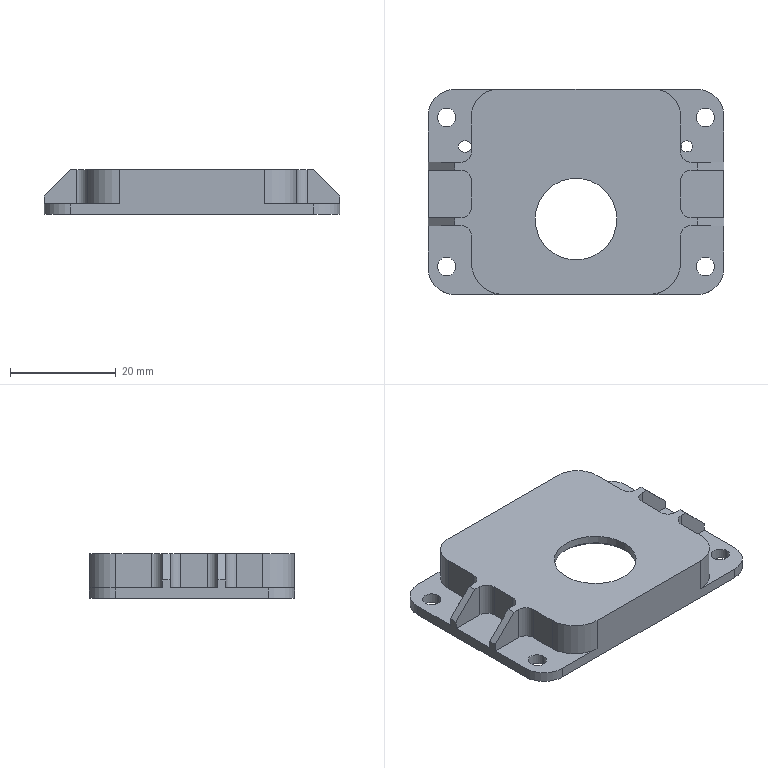NC program | NX | posted with a generic post | part box 56 x 38.85 x 8.5 mm
Lines 2660 to 4316 of 4316:
(ZLEVEL_PROFILE_1 , TOOL : D6R0.5)
N5276 T16 M6
N5278 G54
N5280 G17 G0 G90 X28.022 Y-1.521 S9500 M3
N5282 G43 Z30. H16
N5284 Z2.929
N5286 G94 G1 Z-0.071 F3500.
N5288 G3 X25.776 Y-4.427 R3.
N5290 G1 X25.778 Y-6.715
N5292 X25.775 Y-6.835
N5294 X25.813 Y-6.842 Z-0.106
N5296 X25.846 Y-6.848 Z-0.141
N5298 X25.849 Y-6.715
N5300 X25.848 Y-4.402
N5302 X25.884 Z-0.177
N5304 X25.918 Y-4.401 Z-0.212
N5306 X25.919 Y-4.875
N5308 Y-6.375
N5310 X25.916 Y-6.849
N5312 X25.955 Z-0.247
N5314 X25.987 Z-0.283
N5316 X25.99 Y-6.375
N5318 Y-4.875
N5320 X25.989 Y-4.401
N5322 X26.025 Z-0.318
N5324 X26.06 Y-4.4 Z-0.354
N5326 X26.061 Y-4.875
N5328 Y-6.375
N5330 X26.058 Y-6.85
N5332 X26.096 Z-0.389
N5334 X26.128 Z-0.424
N5336 X26.131 Y-6.375
N5338 Y-4.875
N5340 X26.13 Y-4.4
N5342 X26.167 Z-0.46
N5344 X26.201 Y-4.399 Z-0.495
N5346 X26.202 Y-4.875
N5348 Y-6.375
N5350 X26.199 Y-6.851
N5352 X26.237 Z-0.53
N5354 X26.27 Z-0.566
N5356 X26.273 Y-6.375
N5358 Y-4.875
N5360 X26.272 Y-4.399
N5362 X26.308 Z-0.601
N5364 X26.343 Y-4.398 Z-0.636
N5366 X26.344 Y-4.875
N5368 Y-6.375
N5370 X26.341 Y-6.852
N5372 X26.379 Z-0.672
N5374 X26.411 Z-0.707
N5376 X26.414 Y-6.375
N5378 Y-4.875
N5380 X26.413 Y-4.398
N5382 X26.45 Z-0.742
N5384 X26.484 Y-4.397 Z-0.778
N5386 X26.485 Y-4.875
N5388 Y-6.375
N5390 X26.482 Y-6.853
N5392 X26.52 Z-0.813
N5394 X26.553 Z-0.849
N5396 X26.556 Y-6.375
N5398 Y-4.875
N5400 X26.555 Y-4.397
N5402 X26.591 Z-0.884
N5404 X26.625 Y-4.396 Z-0.919
N5406 X26.626 Y-4.875
N5408 Y-6.375
N5410 X26.623 Y-6.854
N5412 X26.662 Z-0.955
N5414 X26.694 Z-0.99
N5416 X26.697 Y-6.375
N5418 Y-4.875
N5420 X26.696 Y-4.396
N5422 X26.732 Z-1.025
N5424 X26.767 Y-4.395 Z-1.061
N5426 X26.768 Y-4.875
N5428 Y-6.375
N5430 X26.765 Y-6.855
N5432 X26.803 Z-1.096
N5434 X26.838 Z-1.131
N5436 Y-6.375
N5438 Y-4.875
N5440 Y-4.395
N5442 X26.874 Z-1.167
N5444 X26.908 Y-4.394 Z-1.202
N5446 X26.909 Y-4.875
N5448 Y-6.375
N5450 X26.906 Y-6.856
N5452 X26.945 Z-1.237
N5454 X26.977 Z-1.273
N5456 X26.98 Y-6.375
N5458 Y-4.875
N5460 X26.979 Y-4.394
N5462 X27.015 Z-1.308
N5464 X27.05 Y-4.393 Z-1.344
N5466 X27.051 Y-4.875
N5468 Y-6.375
N5470 X27.048 Y-6.856
N5472 X27.086 Y-6.857 Z-1.379
N5474 X27.118 Z-1.414
N5476 X27.121 Y-6.375
N5478 Y-4.875
N5480 Y-4.393
N5482 X27.157 Z-1.45
N5484 X27.191 Z-1.485
N5486 X27.192 Y-4.875
N5488 Y-6.375
N5490 X27.189 Y-6.857
N5492 X27.227 Z-1.52
N5494 X27.26 Z-1.556
N5496 X27.263 Y-6.375
N5498 Y-4.875
N5500 X27.262 Y-4.392
N5502 X27.298 Z-1.591
N5504 X27.333 Z-1.626
N5506 Y-4.875
N5508 Y-6.375
N5510 X27.331 Y-6.858
N5512 X27.369 Z-1.662
N5514 X27.401 Z-1.697
N5516 X27.404 Y-6.375
N5518 Y-4.875
N5520 X27.403 Y-4.392
N5522 X27.44 Z-1.732
N5524 X27.474 Z-1.768
N5526 X27.475 Y-4.875
N5528 Y-6.375
N5530 X27.472 Y-6.858
N5532 X27.51 Z-1.803
N5534 X27.543 Z-1.838
N5536 X27.546 Y-6.375
N5538 Y-4.875
N5540 X27.545 Y-4.392
N5542 X27.581 Y-4.391 Z-1.874
N5544 X27.616 Z-1.909
N5546 Y-4.875
N5548 Y-6.375
N5550 X27.613 Y-6.859
N5552 X27.652 Z-1.945
N5554 X27.684 Z-1.98
N5556 X27.687 Y-6.375
N5558 Y-4.875
N5560 X27.686 Y-4.391
N5562 X27.722 Z-2.015
N5564 X27.757 Z-2.051
N5566 X27.758 Y-4.875
N5568 Y-6.375
N5570 X27.755 Y-6.859
N5572 X27.793 Z-2.086
N5574 X27.826 Z-2.121
N5576 X27.828 Y-6.375
N5578 Y-4.875
N5580 Y-4.391
N5582 X27.864 Z-2.157
N5584 X27.898 Z-2.192
N5586 X27.899 Y-4.875
N5588 Y-6.375
N5590 X27.896 Y-6.86
N5592 X27.934 Z-2.227
N5594 X27.967 Z-2.263
N5596 X27.97 Y-6.375
N5598 Y-4.875
N5600 X27.969 Y-4.39
N5602 X28.005 Z-2.298
N5604 X28.04 Z-2.333
N5606 X28.041 Y-4.875
N5608 Y-6.375
N5610 X28.038 Y-6.86
N5612 X28.076 Z-2.369
N5614 X28.108 Z-2.404
N5616 X28.111 Y-6.375
N5618 Y-4.875
N5620 Y-4.39
N5622 X28.147 Z-2.44
N5624 X28.181 Z-2.475
N5626 X28.182 Y-4.875
N5628 Y-6.375
N5630 X28.179 Y-6.86
N5632 X28.217 Z-2.51
N5634 X28.25 Z-2.546
N5636 X28.253 Y-6.375
N5638 Y-4.875
N5640 X28.252 Y-4.39
N5642 X28.288 Z-2.581
N5644 X28.323 Z-2.616
N5646 Y-4.875
N5648 Y-6.375
N5650 X28.321 Y-6.86
N5652 X28.359 Z-2.652
N5654 X28.391 Z-2.687
N5656 X28.394 Y-6.375
N5658 Y-4.875
N5660 X28.393 Y-4.39
N5662 X28.429 Z-2.722
N5664 X28.464 Z-2.758
N5666 X28.465 Y-4.875
N5668 Y-6.375
N5670 X28.462 Y-6.86
N5672 X28.5 Z-2.793
N5674 X28.533 Z-2.828
N5676 X28.536 Y-6.375
N5678 Y-4.875
N5680 X28.535 Y-4.39
N5682 X28.571 Z-2.864
N5684 X28.605 Z-2.899
N5686 X28.606 Y-4.875
N5688 Y-6.375
N5690 X28.603 Y-6.86
N5692 X28.642 Z-2.934
N5694 X28.674 Z-2.97
N5696 X28.677 Y-6.375
N5698 Y-4.875
N5700 X28.676 Y-4.39
N5702 X28.712 Z-3.005
N5704 X28.747 Z-3.041
N5706 X28.748 Y-4.875
N5708 Y-6.375
N5710 X28.745 Y-6.86
N5712 X28.783 Z-3.076
N5714 X28.815 Y-6.859 Z-3.111
N5716 X28.818 Y-6.375
N5718 Y-4.875
N5720 Y-4.39
N5722 X28.854 Y-4.391 Z-3.147
N5724 X28.888 Z-3.182
N5726 X28.889 Y-4.875
N5728 Y-6.375
N5730 X28.886 Y-6.859
N5732 X28.924 Z-3.217
N5734 X28.957 Z-3.253
N5736 X28.96 Y-6.375
N5738 Y-4.875
N5740 X28.959 Y-4.391
N5742 X28.995 Z-3.288
N5744 X29.03 Z-3.323
N5746 X29.031 Y-4.875
N5748 Y-6.375
N5750 X29.028 Y-6.859
N5752 X29.066 Z-3.359
N5754 X29.098 Z-3.394
N5756 X29.101 Y-6.375
N5758 Y-4.875
N5760 X29.1 Y-4.391
N5762 X29.137 Z-3.429
N5764 X29.171 Y-4.392 Z-3.465
N5766 X29.172 Y-4.875
N5768 Y-6.375
N5770 X29.169 Y-6.858
N5772 X29.207 Z-3.5
N5774 X29.24 Z-3.536
N5776 X29.243 Y-6.375
N5778 Y-4.875
N5780 X29.242 Y-4.392
N5782 X29.278 Z-3.571
N5784 X29.313 Z-3.606
N5786 Y-4.875
N5788 Y-6.375
N5790 X29.31 Y-6.858
N5792 X29.349 Z-3.642
N5794 X29.381 Z-3.677
N5796 X29.384 Y-6.375
N5798 Y-4.875
N5800 X29.383 Y-4.392
N5802 X29.419 Z-3.712
N5804 X29.454 Z-3.748
N5806 X29.455 Y-4.875
N5808 Y-6.375
N5810 X29.452 Y-6.858
N5812 X29.49 Y-6.857 Z-3.783
N5814 X29.523 Z-3.818
N5816 X29.525 Y-6.375
N5818 Y-4.875
N5820 Y-4.393
N5822 X29.561 Z-3.854
N5824 X29.595 Z-3.889
N5826 X29.596 Y-4.875
N5828 Y-6.375
N5830 X29.594 Y-6.857
N5832 X29.632 Z-3.924
N5834 X29.664 Z-3.96
N5836 X29.667 Y-6.375
N5838 Y-4.875
N5840 X29.666 Y-4.393
N5842 X29.702 Y-4.394 Z-3.995
N5844 X29.737 Z-4.031
N5846 X29.738 Y-4.875
N5848 Y-6.375
N5850 X29.735 Y-6.856
N5852 X29.773 Z-4.066
N5854 X29.805 Z-4.101
N5856 X29.808 Y-6.375
N5858 Y-4.875
N5860 X29.807 Y-4.394
N5862 X29.844 Y-4.395 Z-4.137
N5864 X29.878 Z-4.172
N5866 X29.879 Y-4.875
N5868 Y-6.375
N5870 X29.876 Y-6.855
N5872 X29.914 Z-4.207
N5874 X29.947 Z-4.243
N5876 X29.95 Y-6.375
N5878 Y-4.875
N5880 X29.949 Y-4.395
N5882 X29.985 Y-4.396 Z-4.278
N5884 X30.02 Z-4.313
N5886 Y-4.875
N5888 Y-6.375
N5890 X30.018 Y-6.854
N5892 X30.056 Z-4.349
N5894 X30.088 Z-4.384
N5896 X30.091 Y-6.375
N5898 Y-4.875
N5900 X30.09 Y-4.396
N5902 X30.127 Y-4.397 Z-4.419
N5904 X30.161 Z-4.455
N5906 X30.162 Y-4.875
N5908 Y-6.375
N5910 X30.159 Y-6.853
N5912 X30.197 Z-4.49
N5914 X30.23 Z-4.525
N5916 X30.233 Y-6.375
N5918 Y-4.875
N5920 X30.232 Y-4.397
N5922 X30.268 Y-4.398 Z-4.561
N5924 X30.302 Z-4.596
N5926 X30.303 Y-4.875
N5928 Y-6.375
N5930 X30.3 Y-6.852
N5932 X30.339 Z-4.632
N5934 X30.371 Z-4.667
N5936 X30.374 Y-6.375
N5938 Y-4.875
N5940 X30.373 Y-4.398
N5942 X30.409 Y-4.399 Z-4.702
N5944 X30.444 Z-4.738
N5946 X30.445 Y-4.875
N5948 Y-6.375
N5950 X30.442 Y-6.851
N5952 X30.48 Z-4.773
N5954 X30.512 Z-4.808
N5956 X30.515 Y-6.375
N5958 Y-4.875
N5960 Y-4.399
N5962 X30.551 Y-4.4 Z-4.844
N5964 X30.585 Z-4.879
N5966 X30.586 Y-4.875
N5968 Y-6.375
N5970 X30.583 Y-6.85
N5972 X30.622 Z-4.914
N5974 X30.654 Z-4.95
N5976 X30.657 Y-6.375
N5978 Y-4.875
N5980 X30.656 Y-4.401
N5982 X30.692 Z-4.985
N5984 X30.727 Z-5.02
N5986 X30.728 Y-4.875
N5988 Y-6.375
N5990 X30.725 Y-6.849
N5992 X30.763 Z-5.056
N5994 X30.795 Z-5.091
N5996 X30.798 Y-6.375
N5998 Y-4.875
N6000 X30.797 Y-4.402
N6002 X30.834 Z-5.127
N6004 X30.868 Z-5.162
N6006 X30.869 Y-6.715
N6008 X30.866 Y-6.848
N6010 X30.904 Z-5.197
N6012 X30.937 Z-5.233
N6014 X30.94 Y-6.715
N6016 X30.939 Y-4.402
N6018 X31.006 Y-4.445 Z-5.299
N6020 X31.007 Y-6.715
N6022 X31.004 Y-6.825
N6024 X31.072 Y-6.785 Z-5.366
N6026 X31.073 Y-6.715
N6028 Y-4.524
N6030 X31.14 Y-4.603 Z-5.433
N6032 Y-6.744
N6034 G3 X33.422 Y-9.657 R3.
N6036 G1 Z-2.433
N6038 G0 Z30.
N6040 X27.981 Y9.052
N6042 Z2.929
N6044 G1 Z-0.071
N6046 G3 X25.775 Y6.085 R3.
N6048 G1 X25.778 Y5.965
N6050 X25.776 Y3.677
N6052 X25.848 Y3.652 Z-0.141
N6054 X25.849 Y5.965
N6056 X25.846 Y6.098
N6058 X25.884 Z-0.177
N6060 X25.916 Y6.099 Z-0.212
N6062 X25.919 Y5.625
N6064 Y4.125
N6066 X25.918 Y3.651
N6068 X25.955 Z-0.247
N6070 X25.989 Z-0.283
N6072 X25.99 Y4.125
N6074 Y5.625
N6076 X25.987 Y6.099
N6078 X26.025 Z-0.318
N6080 X26.058 Y6.1 Z-0.354
N6082 X26.061 Y5.625
N6084 Y4.125
N6086 X26.06 Y3.65
N6088 X26.096 Z-0.389
N6090 X26.13 Z-0.424
N6092 X26.131 Y4.125
N6094 Y5.625
N6096 X26.128 Y6.1
N6098 X26.167 Z-0.46
N6100 X26.199 Y6.101 Z-0.495
N6102 X26.202 Y5.625
N6104 Y4.125
N6106 X26.201 Y3.649
N6108 X26.237 Z-0.53
N6110 X26.272 Z-0.566
N6112 X26.273 Y4.125
N6114 Y5.625
N6116 X26.27 Y6.101
N6118 X26.308 Z-0.601
N6120 X26.341 Y6.102 Z-0.636
N6122 X26.344 Y5.625
N6124 Y4.125
N6126 X26.343 Y3.648
N6128 X26.379 Z-0.672
N6130 X26.413 Z-0.707
N6132 X26.414 Y4.125
N6134 Y5.625
N6136 X26.411 Y6.102
N6138 X26.45 Z-0.742
N6140 X26.482 Y6.103 Z-0.778
N6142 X26.485 Y5.625
N6144 Y4.125
N6146 X26.484 Y3.647
N6148 X26.52 Z-0.813
N6150 X26.555 Z-0.849
N6152 X26.556 Y4.125
N6154 Y5.625
N6156 X26.553 Y6.103
N6158 X26.591 Z-0.884
N6160 X26.623 Y6.104 Z-0.919
N6162 X26.626 Y5.625
N6164 Y4.125
N6166 X26.625 Y3.646
N6168 X26.662 Z-0.955
N6170 X26.696 Z-0.99
N6172 X26.697 Y4.125
N6174 Y5.625
N6176 X26.694 Y6.104
N6178 X26.732 Z-1.025
N6180 X26.765 Y6.105 Z-1.061
N6182 X26.768 Y5.625
N6184 Y4.125
N6186 X26.767 Y3.645
N6188 X26.803 Z-1.096
N6190 X26.838 Z-1.131
N6192 Y4.125
N6194 Y5.625
N6196 Y6.105
N6198 X26.874 Z-1.167
N6200 X26.906 Y6.106 Z-1.202
N6202 X26.909 Y5.625
N6204 Y4.125
N6206 X26.908 Y3.644
N6208 X26.945 Z-1.237
N6210 X26.979 Z-1.273
N6212 X26.98 Y4.125
N6214 Y5.625
N6216 X26.977 Y6.106
N6218 X27.015 Z-1.308
N6220 X27.048 Z-1.344
N6222 X27.051 Y5.625
N6224 Y4.125
N6226 X27.05 Y3.643
N6228 X27.086 Z-1.379
N6230 X27.121 Z-1.414
N6232 Y4.125
N6234 Y5.625
N6236 X27.118 Y6.107
N6238 X27.157 Z-1.45
N6240 X27.189 Z-1.485
N6242 X27.192 Y5.625
N6244 Y4.125
N6246 X27.191 Y3.643
N6248 X27.227 Y3.642 Z-1.52
N6250 X27.262 Z-1.556
N6252 X27.263 Y4.125
N6254 Y5.625
N6256 X27.26 Y6.108
N6258 X27.298 Z-1.591
N6260 X27.331 Z-1.626
N6262 X27.333 Y5.625
N6264 Y4.125
N6266 Y3.642
N6268 X27.369 Z-1.662
N6270 X27.403 Z-1.697
N6272 X27.404 Y4.125
N6274 Y5.625
N6276 X27.401 Y6.108
N6278 X27.44 Z-1.732
N6280 X27.472 Z-1.768
N6282 X27.475 Y5.625
N6284 Y4.125
N6286 X27.474 Y3.642
N6288 X27.51 Z-1.803
N6290 X27.545 Z-1.838
N6292 X27.546 Y4.125
N6294 Y5.625
N6296 X27.543 Y6.108
N6298 X27.581 Y6.109 Z-1.874
N6300 X27.613 Z-1.909
N6302 X27.616 Y5.625
N6304 Y4.125
N6306 Y3.641
N6308 X27.652 Z-1.945
N6310 X27.686 Z-1.98
N6312 X27.687 Y4.125
N6314 Y5.625
N6316 X27.684 Y6.109
N6318 X27.722 Z-2.015
N6320 X27.755 Z-2.051
N6322 X27.758 Y5.625
N6324 Y4.125
N6326 X27.757 Y3.641
N6328 X27.793 Z-2.086
N6330 X27.828 Z-2.121
N6332 Y4.125
N6334 Y5.625
N6336 X27.826 Y6.109
N6338 X27.864 Z-2.157
N6340 X27.896 Z-2.192
N6342 X27.899 Y5.625
N6344 Y4.125
N6346 X27.898 Y3.64
N6348 X27.934 Z-2.227
N6350 X27.969 Z-2.263
N6352 X27.97 Y4.125
N6354 Y5.625
N6356 X27.967 Y6.11
N6358 X28.005 Z-2.298
N6360 X28.038 Z-2.333
N6362 X28.041 Y5.625
N6364 Y4.125
N6366 X28.04 Y3.64
N6368 X28.076 Z-2.369
N6370 X28.111 Z-2.404
N6372 Y4.125
N6374 Y5.625
N6376 X28.108 Y6.11
N6378 X28.147 Z-2.44
N6380 X28.179 Z-2.475
N6382 X28.182 Y5.625
N6384 Y4.125
N6386 X28.181 Y3.64
N6388 X28.217 Z-2.51
N6390 X28.252 Z-2.546
N6392 X28.253 Y4.125
N6394 Y5.625
N6396 X28.25 Y6.11
N6398 X28.288 Z-2.581
N6400 X28.321 Z-2.616
N6402 X28.323 Y5.625
N6404 Y4.125
N6406 Y3.64
N6408 X28.359 Z-2.652
N6410 X28.393 Z-2.687
N6412 X28.394 Y4.125
N6414 Y5.625
N6416 X28.391 Y6.11
N6418 X28.429 Z-2.722
N6420 X28.462 Z-2.758
N6422 X28.465 Y5.625
N6424 Y4.125
N6426 X28.464 Y3.64
N6428 X28.5 Z-2.793
N6430 X28.535 Z-2.828
N6432 X28.536 Y4.125
N6434 Y5.625
N6436 X28.533 Y6.11
N6438 X28.571 Z-2.864
N6440 X28.603 Z-2.899
N6442 X28.606 Y5.625
N6444 Y4.125
N6446 X28.605 Y3.64
N6448 X28.642 Z-2.934
N6450 X28.676 Z-2.97
N6452 X28.677 Y4.125
N6454 Y5.625
N6456 X28.674 Y6.11
N6458 X28.712 Z-3.005
N6460 X28.745 Z-3.041
N6462 X28.748 Y5.625
N6464 Y4.125
N6466 X28.747 Y3.64
N6468 X28.783 Z-3.076
N6470 X28.818 Y3.641 Z-3.111
N6472 Y4.125
N6474 Y5.625
N6476 X28.815 Y6.109
N6478 X28.854 Z-3.147
N6480 X28.886 Z-3.182
N6482 X28.889 Y5.625
N6484 Y4.125
N6486 X28.888 Y3.641
N6488 X28.924 Z-3.217
N6490 X28.959 Z-3.253
N6492 X28.96 Y4.125
N6494 Y5.625
N6496 X28.957 Y6.109
N6498 X28.995 Z-3.288
N6500 X29.028 Z-3.323
N6502 X29.031 Y5.625
N6504 Y4.125
N6506 X29.03 Y3.641
N6508 X29.066 Z-3.359
N6510 X29.1 Z-3.394
N6512 X29.101 Y4.125
N6514 Y5.625
N6516 X29.098 Y6.109
N6518 X29.137 Y6.108 Z-3.429
N6520 X29.169 Z-3.465
N6522 X29.172 Y5.625
N6524 Y4.125
N6526 X29.171 Y3.642
N6528 X29.207 Z-3.5
N6530 X29.242 Z-3.536
N6532 X29.243 Y4.125
N6534 Y5.625
N6536 X29.24 Y6.108
N6538 X29.278 Z-3.571
N6540 X29.31 Z-3.606
N6542 X29.313 Y5.625
N6544 Y4.125
N6546 Y3.642
N6548 X29.349 Z-3.642
N6550 X29.383 Z-3.677
N6552 X29.384 Y4.125
N6554 Y5.625
N6556 X29.381 Y6.108
N6558 X29.419 Z-3.712
N6560 X29.452 Y6.107 Z-3.748
N6562 X29.455 Y5.625
N6564 Y4.125
N6566 X29.454 Y3.643
N6568 X29.49 Z-3.783
N6570 X29.525 Z-3.818
N6572 Y4.125
N6574 Y5.625
N6576 X29.523 Y6.107
N6578 X29.561 Z-3.854
N6580 X29.594 Z-3.889
N6582 X29.596 Y5.625
N6584 Y4.125
N6586 X29.595 Y3.643
N6588 X29.632 Z-3.924
N6590 X29.666 Z-3.96
N6592 X29.667 Y4.125
N6594 Y5.625
N6596 X29.664 Y6.107
N6598 X29.702 Y6.106 Z-3.995
N6600 X29.735 Z-4.031
N6602 X29.738 Y5.625
N6604 Y4.125
N6606 X29.737 Y3.644
N6608 X29.773 Z-4.066
N6610 X29.807 Z-4.101
N6612 X29.808 Y4.125
N6614 Y5.625
N6616 X29.805 Y6.106
N6618 X29.844 Y6.105 Z-4.137
N6620 X29.876 Z-4.172
N6622 X29.879 Y5.625
N6624 Y4.125
N6626 X29.878 Y3.645
N6628 X29.914 Z-4.207
N6630 X29.949 Z-4.243
N6632 X29.95 Y4.125
N6634 Y5.625
N6636 X29.947 Y6.105
N6638 X29.985 Y6.104 Z-4.278
N6640 X30.018 Z-4.313
N6642 X30.02 Y5.625
N6644 Y4.125
N6646 Y3.646
N6648 X30.056 Z-4.349
N6650 X30.09 Z-4.384
N6652 X30.091 Y4.125
N6654 Y5.625
N6656 X30.088 Y6.104
N6658 X30.127 Y6.103 Z-4.419
N6660 X30.159 Z-4.455
N6662 X30.162 Y5.625
N6664 Y4.125
N6666 X30.161 Y3.647
N6668 X30.197 Z-4.49
N6670 X30.232 Z-4.525
N6672 X30.233 Y4.125
N6674 Y5.625
N6676 X30.23 Y6.102
N6678 X30.268 Z-4.561
N6680 X30.3 Z-4.596
N6682 X30.303 Y5.625
N6684 Y4.125
N6686 X30.302 Y3.648
N6688 X30.339 Z-4.632
N6690 X30.373 Z-4.667
N6692 X30.374 Y4.125
N6694 Y5.625
N6696 X30.371 Y6.101
N6698 X30.409 Z-4.702
N6700 X30.442 Z-4.738
N6702 X30.445 Y5.625
N6704 Y4.125
N6706 X30.444 Y3.649
N6708 X30.48 Z-4.773
N6710 X30.515 Z-4.808
N6712 Y4.125
N6714 Y5.625
N6716 X30.512 Y6.1
N6718 X30.551 Z-4.844
N6720 X30.583 Z-4.879
N6722 X30.586 Y5.625
N6724 Y4.125
N6726 X30.585 Y3.65
N6728 X30.622 Z-4.914
N6730 X30.656 Z-4.95
N6732 X30.657 Y4.125
N6734 Y5.625
N6736 X30.654 Y6.099
N6738 X30.692 Z-4.985
N6740 X30.725 Z-5.02
N6742 X30.728 Y5.625
N6744 Y4.125
N6746 X30.727 Y3.651
N6748 X30.763 Z-5.056
N6750 X30.797 Z-5.091
N6752 X30.798 Y4.125
N6754 Y5.625
N6756 X30.795 Y6.099
N6758 X30.834 Y6.098 Z-5.127
N6760 X30.866 Z-5.162
N6762 X30.869 Y5.965
N6764 X30.868 Y3.652
N6766 X30.904 Z-5.197
N6768 X30.939 Z-5.233
N6770 X30.94 Y5.965
N6772 X30.937 Y6.098
N6774 X31.004 Y6.075 Z-5.299
N6776 X31.007 Y5.965
N6778 X31.006 Y3.695
N6780 X31.073 Y3.774 Z-5.366
N6782 Y5.965
N6784 X31.072 Y6.035
N6786 X31.14 Y5.994 Z-5.433
N6788 Y3.853
N6790 G3 X33.468 Y0.93 R3.
N6792 G1 Z-2.433
N6794 G0 Z30.
N6796 X-28.022 Y0.771
N6798 Z2.929
N6800 G1 Z-0.071
N6802 G3 X-25.776 Y3.677 R3.
N6804 G1 X-25.778 Y5.965
N6806 X-25.775 Y6.085
N6808 X-25.813 Y6.092 Z-0.106
N6810 X-25.846 Y6.098 Z-0.141
N6812 X-25.849 Y5.965
N6814 X-25.848 Y3.652
N6816 X-25.884 Z-0.177
N6818 X-25.918 Y3.651 Z-0.212
N6820 X-25.919 Y4.125
N6822 Y5.625
N6824 X-25.916 Y6.099
N6826 X-25.955 Z-0.247
N6828 X-25.987 Z-0.283
N6830 X-25.99 Y5.625
N6832 Y4.125
N6834 X-25.989 Y3.651
N6836 X-26.025 Z-0.318
N6838 X-26.06 Y3.65 Z-0.354
N6840 X-26.061 Y4.125
N6842 Y5.625
N6844 X-26.058 Y6.1
N6846 X-26.096 Z-0.389
N6848 X-26.128 Z-0.424
N6850 X-26.131 Y5.625
N6852 Y4.125
N6854 X-26.13 Y3.65
N6856 X-26.167 Z-0.46
N6858 X-26.201 Y3.649 Z-0.495
N6860 X-26.202 Y4.125
N6862 Y5.625
N6864 X-26.199 Y6.101
N6866 X-26.237 Z-0.53
N6868 X-26.27 Z-0.566
N6870 X-26.273 Y5.625
N6872 Y4.125
N6874 X-26.272 Y3.649
N6876 X-26.308 Z-0.601
N6878 X-26.343 Y3.648 Z-0.636
N6880 X-26.344 Y4.125
N6882 Y5.625
N6884 X-26.341 Y6.102
N6886 X-26.379 Z-0.672
N6888 X-26.411 Z-0.707
N6890 X-26.414 Y5.625
N6892 Y4.125
N6894 X-26.413 Y3.648
N6896 X-26.45 Z-0.742
N6898 X-26.484 Y3.647 Z-0.778
N6900 X-26.485 Y4.125
N6902 Y5.625
N6904 X-26.482 Y6.103
N6906 X-26.52 Z-0.813
N6908 X-26.553 Z-0.849
N6910 X-26.556 Y5.625
N6912 Y4.125
N6914 X-26.555 Y3.647
N6916 X-26.591 Z-0.884
N6918 X-26.625 Y3.646 Z-0.919
N6920 X-26.626 Y4.125
N6922 Y5.625
N6924 X-26.623 Y6.104
N6926 X-26.662 Z-0.955
N6928 X-26.694 Z-0.99
N6930 X-26.697 Y5.625
N6932 Y4.125
N6934 X-26.696 Y3.646
N6936 X-26.732 Z-1.025
N6938 X-26.767 Y3.645 Z-1.061
N6940 X-26.768 Y4.125
N6942 Y5.625
N6944 X-26.765 Y6.105
N6946 X-26.803 Z-1.096
N6948 X-26.838 Z-1.131
N6950 Y5.625
N6952 Y4.125
N6954 Y3.645
N6956 X-26.874 Z-1.167
N6958 X-26.908 Y3.644 Z-1.202
N6960 X-26.909 Y4.125
N6962 Y5.625
N6964 X-26.906 Y6.106
N6966 X-26.945 Z-1.237
N6968 X-26.977 Z-1.273
N6970 X-26.98 Y5.625
N6972 Y4.125
N6974 X-26.979 Y3.644
N6976 X-27.015 Z-1.308
N6978 X-27.05 Y3.643 Z-1.344
N6980 X-27.051 Y4.125
N6982 Y5.625
N6984 X-27.048 Y6.106
N6986 X-27.086 Y6.107 Z-1.379
N6988 X-27.118 Z-1.414
N6990 X-27.121 Y5.625
N6992 Y4.125
N6994 Y3.643
N6996 X-27.157 Z-1.45
N6998 X-27.191 Z-1.485
N7000 X-27.192 Y4.125
N7002 Y5.625
N7004 X-27.189 Y6.107
N7006 X-27.227 Z-1.52
N7008 X-27.26 Y6.108 Z-1.556
N7010 X-27.263 Y5.625
N7012 Y4.125
N7014 X-27.262 Y3.642
N7016 X-27.298 Z-1.591
N7018 X-27.333 Z-1.626
N7020 Y4.125
N7022 Y5.625
N7024 X-27.331 Y6.108
N7026 X-27.369 Z-1.662
N7028 X-27.401 Z-1.697
N7030 X-27.404 Y5.625
N7032 Y4.125
N7034 X-27.403 Y3.642
N7036 X-27.44 Z-1.732
N7038 X-27.474 Z-1.768
N7040 X-27.475 Y4.125
N7042 Y5.625
N7044 X-27.472 Y6.108
N7046 X-27.51 Z-1.803
N7048 X-27.543 Z-1.838
N7050 X-27.546 Y5.625
N7052 Y4.125
N7054 X-27.545 Y3.642
N7056 X-27.581 Y3.641 Z-1.874
N7058 X-27.616 Z-1.909
N7060 Y4.125
N7062 Y5.625
N7064 X-27.613 Y6.109
N7066 X-27.652 Z-1.945
N7068 X-27.684 Z-1.98
N7070 X-27.687 Y5.625
N7072 Y4.125
N7074 X-27.686 Y3.641
N7076 X-27.722 Z-2.015
N7078 X-27.757 Z-2.051
N7080 X-27.758 Y4.125
N7082 Y5.625
N7084 X-27.755 Y6.109
N7086 X-27.793 Z-2.086
N7088 X-27.826 Z-2.121
N7090 X-27.828 Y5.625
N7092 Y4.125
N7094 Y3.641
N7096 X-27.864 Z-2.157
N7098 X-27.898 Y3.64 Z-2.192
N7100 X-27.899 Y4.125
N7102 Y5.625
N7104 X-27.896 Y6.109
N7106 X-27.934 Y6.11 Z-2.227
N7108 X-27.967 Z-2.263
N7110 X-27.97 Y5.625
N7112 Y4.125
N7114 X-27.969 Y3.64
N7116 X-28.005 Z-2.298
N7118 X-28.04 Z-2.333
N7120 X-28.041 Y4.125
N7122 Y5.625
N7124 X-28.038 Y6.11
N7126 X-28.076 Z-2.369
N7128 X-28.108 Z-2.404
N7130 X-28.111 Y5.625
N7132 Y4.125
N7134 Y3.64
N7136 X-28.147 Z-2.44
N7138 X-28.181 Z-2.475
N7140 X-28.182 Y4.125
N7142 Y5.625
N7144 X-28.179 Y6.11
N7146 X-28.217 Z-2.51
N7148 X-28.25 Z-2.546
N7150 X-28.253 Y5.625
N7152 Y4.125
N7154 X-28.252 Y3.64
N7156 X-28.288 Z-2.581
N7158 X-28.323 Z-2.616
N7160 Y4.125
N7162 Y5.625
N7164 X-28.321 Y6.11
N7166 X-28.359 Z-2.652
N7168 X-28.391 Z-2.687
N7170 X-28.394 Y5.625
N7172 Y4.125
N7174 X-28.393 Y3.64
N7176 X-28.429 Z-2.722
N7178 X-28.464 Z-2.758
N7180 X-28.465 Y4.125
N7182 Y5.625
N7184 X-28.462 Y6.11
N7186 X-28.5 Z-2.793
N7188 X-28.533 Z-2.828
N7190 X-28.536 Y5.625
N7192 Y4.125
N7194 X-28.535 Y3.64
N7196 X-28.571 Z-2.864
N7198 X-28.605 Z-2.899
N7200 X-28.606 Y4.125
N7202 Y5.625
N7204 X-28.603 Y6.11
N7206 X-28.642 Z-2.934
N7208 X-28.674 Z-2.97
N7210 X-28.677 Y5.625
N7212 Y4.125
N7214 X-28.676 Y3.64
N7216 X-28.712 Z-3.005
N7218 X-28.747 Z-3.041
N7220 X-28.748 Y4.125
N7222 Y5.625
N7224 X-28.745 Y6.11
N7226 X-28.783 Z-3.076
N7228 X-28.815 Y6.109 Z-3.111
N7230 X-28.818 Y5.625
N7232 Y4.125
N7234 Y3.641
N7236 X-28.854 Z-3.147
N7238 X-28.888 Z-3.182
N7240 X-28.889 Y4.125
N7242 Y5.625
N7244 X-28.886 Y6.109
N7246 X-28.924 Z-3.217
N7248 X-28.957 Z-3.253
N7250 X-28.96 Y5.625
N7252 Y4.125
N7254 X-28.959 Y3.641
N7256 X-28.995 Z-3.288
N7258 X-29.03 Z-3.323
N7260 X-29.031 Y4.125
N7262 Y5.625
N7264 X-29.028 Y6.109
N7266 X-29.066 Z-3.359
N7268 X-29.098 Z-3.394
N7270 X-29.101 Y5.625
N7272 Y4.125
N7274 X-29.1 Y3.641
N7276 X-29.137 Y3.642 Z-3.429
N7278 X-29.171 Z-3.465
N7280 X-29.172 Y4.125
N7282 Y5.625
N7284 X-29.169 Y6.108
N7286 X-29.207 Z-3.5
N7288 X-29.24 Z-3.536
N7290 X-29.243 Y5.625
N7292 Y4.125
N7294 X-29.242 Y3.642
N7296 X-29.278 Z-3.571
N7298 X-29.313 Z-3.606
N7300 Y4.125
N7302 Y5.625
N7304 X-29.31 Y6.108
N7306 X-29.349 Z-3.642
N7308 X-29.381 Z-3.677
N7310 X-29.384 Y5.625
N7312 Y4.125
N7314 X-29.383 Y3.642
N7316 X-29.419 Z-3.712
N7318 X-29.454 Y3.643 Z-3.748
N7320 X-29.455 Y4.125
N7322 Y5.625
N7324 X-29.452 Y6.107
N7326 X-29.49 Z-3.783
N7328 X-29.523 Z-3.818
N7330 X-29.525 Y5.625
N7332 Y4.125
N7334 Y3.643
N7336 X-29.561 Z-3.854
N7338 X-29.595 Z-3.889
N7340 X-29.596 Y4.125
N7342 Y5.625
N7344 X-29.594 Y6.107
N7346 X-29.632 Z-3.924
N7348 X-29.664 Z-3.96
N7350 X-29.667 Y5.625
N7352 Y4.125
N7354 X-29.666 Y3.643
N7356 X-29.702 Y3.644 Z-3.995
N7358 X-29.737 Z-4.031
N7360 X-29.738 Y4.125
N7362 Y5.625
N7364 X-29.735 Y6.106
N7366 X-29.773 Z-4.066
N7368 X-29.805 Z-4.101
N7370 X-29.808 Y5.625
N7372 Y4.125
N7374 X-29.807 Y3.644
N7376 X-29.844 Y3.645 Z-4.137
N7378 X-29.878 Z-4.172
N7380 X-29.879 Y4.125
N7382 Y5.625
N7384 X-29.876 Y6.105
N7386 X-29.914 Z-4.207
N7388 X-29.947 Z-4.243
N7390 X-29.95 Y5.625
N7392 Y4.125
N7394 X-29.949 Y3.645
N7396 X-29.985 Y3.646 Z-4.278
N7398 X-30.02 Z-4.313
N7400 Y4.125
N7402 Y5.625
N7404 X-30.018 Y6.104
N7406 X-30.056 Z-4.349
N7408 X-30.088 Z-4.384
N7410 X-30.091 Y5.625
N7412 Y4.125
N7414 X-30.09 Y3.646
N7416 X-30.127 Y3.647 Z-4.419
N7418 X-30.161 Z-4.455
N7420 X-30.162 Y4.125
N7422 Y5.625
N7424 X-30.159 Y6.103
N7426 X-30.197 Z-4.49
N7428 X-30.23 Y6.102 Z-4.525
N7430 X-30.233 Y5.625
N7432 Y4.125
N7434 X-30.232 Y3.647
N7436 X-30.268 Y3.648 Z-4.561
N7438 X-30.302 Z-4.596
N7440 X-30.303 Y4.125
N7442 Y5.625
N7444 X-30.3 Y6.102
N7446 X-30.339 Z-4.632
N7448 X-30.371 Y6.101 Z-4.667
N7450 X-30.374 Y5.625
N7452 Y4.125
N7454 X-30.373 Y3.648
N7456 X-30.409 Y3.649 Z-4.702
N7458 X-30.444 Z-4.738
N7460 X-30.445 Y4.125
N7462 Y5.625
N7464 X-30.442 Y6.101
N7466 X-30.48 Z-4.773
N7468 X-30.512 Y6.1 Z-4.808
N7470 X-30.515 Y5.625
N7472 Y4.125
N7474 Y3.649
N7476 X-30.551 Y3.65 Z-4.844
N7478 X-30.585 Z-4.879
N7480 X-30.586 Y4.125
N7482 Y5.625
N7484 X-30.583 Y6.1
N7486 X-30.622 Z-4.914
N7488 X-30.654 Y6.099 Z-4.95
N7490 X-30.657 Y5.625
N7492 Y4.125
N7494 X-30.656 Y3.65
N7496 X-30.692 Y3.651 Z-4.985
N7498 X-30.727 Z-5.02
N7500 X-30.728 Y4.125
N7502 Y5.625
N7504 X-30.725 Y6.099
N7506 X-30.763 Z-5.056
N7508 X-30.795 Z-5.091
N7510 X-30.798 Y5.625
N7512 Y4.125
N7514 X-30.797 Y3.651
N7516 X-30.834 Y3.652 Z-5.127
N7518 X-30.868 Z-5.162
N7520 X-30.869 Y5.965
N7522 X-30.866 Y6.098
N7524 X-30.904 Z-5.197
N7526 X-30.937 Z-5.233
N7528 X-30.94 Y5.965
N7530 X-30.939 Y3.652
N7532 X-31.006 Y3.695 Z-5.299
N7534 X-31.007 Y5.965
N7536 X-31.004 Y6.075
N7538 X-31.072 Y6.035 Z-5.366
N7540 X-31.073 Y5.965
N7542 Y3.774
N7544 X-31.14 Y3.853 Z-5.433
N7546 Y5.994
N7548 G3 X-33.422 Y8.907 R3.
N7550 G1 Z-2.433
N7552 G0 Z30.
N7554 X-27.981 Y-9.802
N7556 Z2.929
N7558 G1 Z-0.071
N7560 G3 X-25.775 Y-6.835 R3.
N7562 G1 X-25.778 Y-6.715
N7564 X-25.776 Y-4.427
N7566 X-25.848 Y-4.402 Z-0.141
N7568 X-25.849 Y-6.715
N7570 X-25.846 Y-6.848
N7572 X-25.884 Z-0.177
N7574 X-25.916 Y-6.849 Z-0.212
N7576 X-25.919 Y-6.375
N7578 Y-4.875
N7580 X-25.918 Y-4.401
N7582 X-25.955 Z-0.247
N7584 X-25.989 Z-0.283
N7586 X-25.99 Y-4.875
N7588 Y-6.375
N7590 X-25.987 Y-6.849
N7592 X-26.025 Z-0.318
N7594 X-26.058 Y-6.85 Z-0.354
N7596 X-26.061 Y-6.375
N7598 Y-4.875
N7600 X-26.06 Y-4.4
N7602 X-26.096 Z-0.389
N7604 X-26.13 Z-0.424
N7606 X-26.131 Y-4.875
N7608 Y-6.375
N7610 X-26.128 Y-6.85
N7612 X-26.167 Z-0.46
N7614 X-26.199 Y-6.851 Z-0.495
N7616 X-26.202 Y-6.375
N7618 Y-4.875
N7620 X-26.201 Y-4.399
N7622 X-26.237 Z-0.53
N7624 X-26.272 Z-0.566
N7626 X-26.273 Y-4.875
N7628 Y-6.375
N7630 X-26.27 Y-6.851
N7632 X-26.308 Z-0.601
N7634 X-26.341 Y-6.852 Z-0.636
N7636 X-26.344 Y-6.375
N7638 Y-4.875
N7640 X-26.343 Y-4.398
N7642 X-26.379 Z-0.672
N7644 X-26.413 Z-0.707
N7646 X-26.414 Y-4.875
N7648 Y-6.375
N7650 X-26.411 Y-6.852
N7652 X-26.45 Z-0.742
N7654 X-26.482 Y-6.853 Z-0.778
N7656 X-26.485 Y-6.375
N7658 Y-4.875
N7660 X-26.484 Y-4.397
N7662 X-26.52 Z-0.813
N7664 X-26.555 Z-0.849
N7666 X-26.556 Y-4.875
N7668 Y-6.375
N7670 X-26.553 Y-6.853
N7672 X-26.591 Z-0.884
N7674 X-26.623 Y-6.854 Z-0.919
N7676 X-26.626 Y-6.375
N7678 Y-4.875
N7680 X-26.625 Y-4.396
N7682 X-26.662 Z-0.955
N7684 X-26.696 Z-0.99
N7686 X-26.697 Y-4.875
N7688 Y-6.375
N7690 X-26.694 Y-6.854
N7692 X-26.732 Z-1.025
N7694 X-26.765 Y-6.855 Z-1.061
N7696 X-26.768 Y-6.375
N7698 Y-4.875
N7700 X-26.767 Y-4.395
N7702 X-26.803 Z-1.096
N7704 X-26.838 Z-1.131
N7706 Y-4.875
N7708 Y-6.375
N7710 Y-6.855
N7712 X-26.874 Z-1.167
N7714 X-26.906 Y-6.856 Z-1.202
N7716 X-26.909 Y-6.375
N7718 Y-4.875
N7720 X-26.908 Y-4.394
N7722 X-26.945 Z-1.237
N7724 X-26.979 Z-1.273
N7726 X-26.98 Y-4.875
N7728 Y-6.375
N7730 X-26.977 Y-6.856
N7732 X-27.015 Z-1.308
N7734 X-27.048 Z-1.344
N7736 X-27.051 Y-6.375
N7738 Y-4.875
N7740 X-27.05 Y-4.393
N7742 X-27.086 Z-1.379
N7744 X-27.121 Z-1.414
N7746 Y-4.875
N7748 Y-6.375
N7750 X-27.118 Y-6.857
N7752 X-27.157 Z-1.45
N7754 X-27.189 Z-1.485
N7756 X-27.192 Y-6.375
N7758 Y-4.875
N7760 X-27.191 Y-4.393
N7762 X-27.227 Z-1.52
N7764 X-27.262 Y-4.392 Z-1.556
N7766 X-27.263 Y-4.875
N7768 Y-6.375
N7770 X-27.26 Y-6.857
N7772 X-27.298 Y-6.858 Z-1.591
N7774 X-27.331 Z-1.626
N7776 X-27.333 Y-6.375
N7778 Y-4.875
N7780 Y-4.392
N7782 X-27.369 Z-1.662
N7784 X-27.403 Z-1.697
N7786 X-27.404 Y-4.875
N7788 Y-6.375
N7790 X-27.401 Y-6.858
N7792 X-27.44 Z-1.732
N7794 X-27.472 Z-1.768
N7796 X-27.475 Y-6.375
N7798 Y-4.875
N7800 X-27.474 Y-4.392
N7802 X-27.51 Z-1.803
N7804 X-27.545 Z-1.838
N7806 X-27.546 Y-4.875
N7808 Y-6.375
N7810 X-27.543 Y-6.858
N7812 X-27.581 Y-6.859 Z-1.874
N7814 X-27.613 Z-1.909
N7816 X-27.616 Y-6.375
N7818 Y-4.875
N7820 Y-4.391
N7822 X-27.652 Z-1.945
N7824 X-27.686 Z-1.98
N7826 X-27.687 Y-4.875
N7828 Y-6.375
N7830 X-27.684 Y-6.859
N7832 X-27.722 Z-2.015
N7834 X-27.755 Z-2.051
N7836 X-27.758 Y-6.375
N7838 Y-4.875
N7840 X-27.757 Y-4.391
N7842 X-27.793 Z-2.086
N7844 X-27.828 Z-2.121
N7846 Y-4.875
N7848 Y-6.375
N7850 X-27.826 Y-6.859
N7852 X-27.864 Z-2.157
N7854 X-27.896 Y-6.86 Z-2.192
N7856 X-27.899 Y-6.375
N7858 Y-4.875
N7860 X-27.898 Y-4.391
N7862 X-27.934 Y-4.39 Z-2.227
N7864 X-27.969 Z-2.263
N7866 X-27.97 Y-4.875
N7868 Y-6.375
N7870 X-27.967 Y-6.86
N7872 X-28.005 Z-2.298
N7874 X-28.038 Z-2.333
N7876 X-28.041 Y-6.375
N7878 Y-4.875
N7880 X-28.04 Y-4.39
N7882 X-28.076 Z-2.369
N7884 X-28.111 Z-2.404
N7886 Y-4.875
N7888 Y-6.375
N7890 X-28.108 Y-6.86
N7892 X-28.147 Z-2.44
N7894 X-28.179 Z-2.475
N7896 X-28.182 Y-6.375
N7898 Y-4.875
N7900 X-28.181 Y-4.39
N7902 X-28.217 Z-2.51
N7904 X-28.252 Z-2.546
N7906 X-28.253 Y-4.875
N7908 Y-6.375
N7910 X-28.25 Y-6.86
N7912 X-28.288 Z-2.581
N7914 X-28.321 Z-2.616
N7916 X-28.323 Y-6.375
N7918 Y-4.875
N7920 Y-4.39
N7922 X-28.359 Z-2.652
N7924 X-28.393 Z-2.687
N7926 X-28.394 Y-4.875
N7928 Y-6.375
N7930 X-28.391 Y-6.86
N7932 X-28.429 Z-2.722
N7934 X-28.462 Z-2.758
N7936 X-28.465 Y-6.375
N7938 Y-4.875
N7940 X-28.464 Y-4.39
N7942 X-28.5 Z-2.793
N7944 X-28.535 Z-2.828
N7946 X-28.536 Y-4.875
N7948 Y-6.375
N7950 X-28.533 Y-6.86
N7952 X-28.571 Z-2.864
N7954 X-28.603 Z-2.899
N7956 X-28.606 Y-6.375
N7958 Y-4.875
N7960 X-28.605 Y-4.39
N7962 X-28.642 Z-2.934
N7964 X-28.676 Z-2.97
N7966 X-28.677 Y-4.875
N7968 Y-6.375
N7970 X-28.674 Y-6.86
N7972 X-28.712 Z-3.005
N7974 X-28.745 Z-3.041
N7976 X-28.748 Y-6.375
N7978 Y-4.875
N7980 X-28.747 Y-4.39
N7982 X-28.783 Z-3.076
N7984 X-28.818 Z-3.111
N7986 Y-4.875
N7988 Y-6.375
N7990 X-28.815 Y-6.859
N7992 X-28.854 Z-3.147
N7994 X-28.886 Z-3.182
N7996 X-28.889 Y-6.375
N7998 Y-4.875
N8000 X-28.888 Y-4.391
N8002 X-28.924 Z-3.217
N8004 X-28.959 Z-3.253
N8006 X-28.96 Y-4.875
N8008 Y-6.375
N8010 X-28.957 Y-6.859
N8012 X-28.995 Z-3.288
N8014 X-29.028 Z-3.323
N8016 X-29.031 Y-6.375
N8018 Y-4.875
N8020 X-29.03 Y-4.391
N8022 X-29.066 Z-3.359
N8024 X-29.1 Z-3.394
N8026 X-29.101 Y-4.875
N8028 Y-6.375
N8030 X-29.098 Y-6.859
N8032 X-29.137 Y-6.858 Z-3.429
N8034 X-29.169 Z-3.465
N8036 X-29.172 Y-6.375
N8038 Y-4.875
N8040 X-29.171 Y-4.392
N8042 X-29.207 Z-3.5
N8044 X-29.242 Z-3.536
N8046 X-29.243 Y-4.875
N8048 Y-6.375
N8050 X-29.24 Y-6.858
N8052 X-29.278 Z-3.571
N8054 X-29.31 Z-3.606
N8056 X-29.313 Y-6.375
N8058 Y-4.875
N8060 Y-4.392
N8062 X-29.349 Z-3.642
N8064 X-29.383 Z-3.677
N8066 X-29.384 Y-4.875
N8068 Y-6.375
N8070 X-29.381 Y-6.858
N8072 X-29.419 Z-3.712
N8074 X-29.452 Z-3.748
N8076 X-29.455 Y-6.375
N8078 Y-4.875
N8080 X-29.454 Y-4.392
N8082 X-29.49 Y-4.393 Z-3.783
N8084 X-29.525 Z-3.818
N8086 Y-4.875
N8088 Y-6.375
N8090 X-29.523 Y-6.857
N8092 X-29.561 Z-3.854
N8094 X-29.594 Z-3.889
N8096 X-29.596 Y-6.375
N8098 Y-4.875
N8100 X-29.595 Y-4.393
N8102 X-29.632 Z-3.924
N8104 X-29.666 Z-3.96
N8106 X-29.667 Y-4.875
N8108 Y-6.375
N8110 X-29.664 Y-6.857
N8112 X-29.702 Y-6.856 Z-3.995
N8114 X-29.735 Z-4.031
N8116 X-29.738 Y-6.375
N8118 Y-4.875
N8120 X-29.737 Y-4.394
N8122 X-29.773 Z-4.066
N8124 X-29.807 Z-4.101
N8126 X-29.808 Y-4.875
N8128 Y-6.375
N8130 X-29.805 Y-6.856
N8132 X-29.844 Y-6.855 Z-4.137
N8134 X-29.876 Z-4.172
N8136 X-29.879 Y-6.375
N8138 Y-4.875
N8140 X-29.878 Y-4.395
N8142 X-29.914 Z-4.207
N8144 X-29.949 Z-4.243
N8146 X-29.95 Y-4.875
N8148 Y-6.375
N8150 X-29.947 Y-6.855
N8152 X-29.985 Y-6.854 Z-4.278
N8154 X-30.018 Z-4.313
N8156 X-30.02 Y-6.375
N8158 Y-4.875
N8160 Y-4.396
N8162 X-30.056 Z-4.349
N8164 X-30.09 Z-4.384
N8166 X-30.091 Y-4.875
N8168 Y-6.375
N8170 X-30.088 Y-6.854
N8172 X-30.127 Y-6.853 Z-4.419
N8174 X-30.159 Z-4.455
N8176 X-30.162 Y-6.375
N8178 Y-4.875
N8180 X-30.161 Y-4.397
N8182 X-30.197 Z-4.49
N8184 X-30.232 Z-4.525
N8186 X-30.233 Y-4.875
N8188 Y-6.375
N8190 X-30.23 Y-6.853
N8192 X-30.268 Y-6.852 Z-4.561
N8194 X-30.3 Z-4.596
N8196 X-30.303 Y-6.375
N8198 Y-4.875
N8200 X-30.302 Y-4.398
N8202 X-30.339 Z-4.632
N8204 X-30.373 Z-4.667
N8206 X-30.374 Y-4.875
N8208 Y-6.375
N8210 X-30.371 Y-6.852
N8212 X-30.409 Y-6.851 Z-4.702
N8214 X-30.442 Z-4.738
N8216 X-30.445 Y-6.375
N8218 Y-4.875
N8220 X-30.444 Y-4.399
N8222 X-30.48 Z-4.773
N8224 X-30.515 Z-4.808
N8226 Y-4.875
N8228 Y-6.375
N8230 X-30.512 Y-6.851
N8232 X-30.551 Y-6.85 Z-4.844
N8234 X-30.583 Z-4.879
N8236 X-30.586 Y-6.375
N8238 Y-4.875
N8240 X-30.585 Y-4.4
N8242 X-30.622 Z-4.914
N8244 X-30.656 Y-4.401 Z-4.95
N8246 X-30.657 Y-4.875
N8248 Y-6.375
N8250 X-30.654 Y-6.85
N8252 X-30.692 Y-6.849 Z-4.985
N8254 X-30.725 Z-5.02
N8256 X-30.728 Y-6.375
N8258 Y-4.875
N8260 X-30.727 Y-4.401
N8262 X-30.763 Z-5.056
N8264 X-30.797 Y-4.402 Z-5.091
N8266 X-30.798 Y-4.875
N8268 Y-6.375
N8270 X-30.795 Y-6.849
N8272 X-30.834 Y-6.848 Z-5.127
N8274 X-30.866 Z-5.162
N8276 X-30.869 Y-6.715
N8278 X-30.868 Y-4.402
N8280 X-30.904 Z-5.197
N8282 X-30.939 Z-5.233
N8284 X-30.94 Y-6.715
N8286 X-30.937 Y-6.848
N8288 X-31.004 Y-6.825 Z-5.299
N8290 X-31.007 Y-6.715
N8292 X-31.006 Y-4.445
N8294 X-31.073 Y-4.524 Z-5.366
N8296 Y-6.715
N8298 X-31.072 Y-6.785
N8300 X-31.14 Y-6.744 Z-5.433
N8302 Y-4.603
N8304 G3 X-33.467 Y-1.68 R3.
N8306 G1 Z-2.433
N8308 G0 Z30.
N8310 M5
(PLANAR_MILL_COPY_COPY_COPY_COPY_COPY_COPY_1_COPY_1 , TOOL : D6A45)
N8312 T01 M6
N8314 G54
N8316 G17 G0 G90 X-0.866 Y20.725 S9500 M3
N8318 G43 Z30. H1
N8320 Z0.5
N8322 G94 G1 Z-1. F1250.
N8324 G3 X0. Y20.225 R1.
N8326 G1 X14.8
N8328 G2 X20.6 Y14.425 R5.8
N8330 G1 Y7.625
N8332 G3 X21.8 Y6.425 R1.2
N8334 G1 X28.
N8336 G2 X28.8 Y5.625 R0.8
N8338 G1 Y4.125
N8340 G2 X28. Y3.325 R0.8
N8342 G1 X21.8
N8344 G3 X20.6 Y2.125 R1.2
N8346 G1 Y-2.875
N8348 G3 X21.8 Y-4.075 R1.2
N8350 G1 X28.
N8352 G2 X28.8 Y-4.875 R0.8
N8354 G1 Y-6.375
N8356 G2 X28. Y-7.175 R0.8
N8358 G1 X21.8
N8360 G3 X20.6 Y-8.375 R1.2
N8362 G1 Y-13.425
N8364 G2 X13.8 Y-20.225 R6.8
N8366 G1 X-13.8
N8368 G2 X-20.6 Y-13.425 R6.8
N8370 G1 Y-8.375
N8372 G3 X-21.8 Y-7.175 R1.2
N8374 G1 X-28.
N8376 G2 X-28.8 Y-6.375 R0.8
N8378 G1 Y-4.875
N8380 G2 X-28. Y-4.075 R0.8
N8382 G1 X-21.8
N8384 G3 X-20.6 Y-2.875 R1.2
N8386 G1 Y2.125
N8388 G3 X-21.8 Y3.325 R1.2
N8390 G1 X-28.
N8392 G2 X-28.8 Y4.125 R0.8
N8394 G1 Y5.625
N8396 G2 X-28. Y6.425 R0.8
N8398 G1 X-21.8
N8400 G3 X-20.6 Y7.625 R1.2
N8402 G1 Y14.425
N8404 G2 X-14.8 Y20.225 R5.8
N8406 G1 X0.
N8408 G3 X0.866 Y20.725 R1.
N8410 G1 Z0.5
N8412 G0 Z30.
N8414 X-0.866 Y-11.598
N8416 Z0.5
N8418 G1 Z-1.
N8420 G3 X0. Y-12.098 R1.
N8422 X6.95 Y-5.148 R6.95
N8424 X0. Y-12.098 R-6.95
N8426 X0.866 Y-11.598 R1.
N8428 G1 Z0.5
N8430 G0 Z30.
(PLANAR_MILL_COPY_COPY_COPY_COPY_COPY_COPY_1_COPY_1_COPY , TOOL : D6A45)
N8432 X20.998 Y21.887
N8434 Z-6.
N8436 G1 Z-7.5
N8438 X20.788 Y21.199
N8440 G3 X21.014 Y20.225 R1.
N8442 G1 X23.
N8444 G2 X28.8 Y14.425 R5.8
N8446 G1 Y9.032
N8448 G3 X29.757 Y9.321 R1.
N8450 G1 X30.191 Y9.783
N8452 Z-6.
N8454 G0 Z30.
N8456 Y-0.033
N8458 Z-6.
N8460 G1 Z-7.5
N8462 X29.757 Y0.429
N8464 G3 X28.8 Y0.718 R1.
N8466 G1 Y-1.468
N8468 G3 X29.757 Y-1.179 R1.
N8470 G1 X30.191 Y-0.717
N8472 Z-6.
N8474 G0 Z30.
N8476 Y-10.533
N8478 Z-6.
N8480 G1 Z-7.5
N8482 X29.757 Y-10.071
N8484 G3 X28.8 Y-9.782 R1.
N8486 G1 Y-14.425
N8488 G2 X23. Y-20.225 R5.8
N8490 G1 X20.434
N8492 G3 X20.163 Y-21.188 R1.
N8494 G1 X20.343 Y-21.892
N8496 Z-6.
N8498 G0 Z30.
N8500 X-20.343
N8502 Z-6.
N8504 G1 Z-7.5
N8506 X-20.163 Y-21.188
N8508 G3 X-20.434 Y-20.225 R1.
N8510 G1 X-23.
N8512 G2 X-28.8 Y-14.425 R5.8
N8514 G1 Y-9.782
N8516 G3 X-29.757 Y-10.071 R1.
N8518 G1 X-30.191 Y-10.533
N8520 Z-6.
N8522 G0 Z30.
N8524 Y-0.717
N8526 Z-6.
N8528 G1 Z-7.5
N8530 X-29.757 Y-1.179
N8532 G3 X-28.8 Y-1.468 R1.
N8534 G1 Y0.718
N8536 G3 X-29.757 Y0.429 R1.
N8538 G1 X-30.191 Y-0.033
N8540 Z-6.
N8542 G0 Z30.
N8544 Y9.783
N8546 Z-6.
N8548 G1 Z-7.5
N8550 X-29.757 Y9.321
N8552 G3 X-28.8 Y9.032 R1.
N8554 G1 Y14.425
N8556 G2 X-23. Y20.225 R5.8
N8558 G1 X-21.014
N8560 G3 X-20.788 Y21.199 R1.
N8562 G1 X-20.998 Y21.887
N8564 Z-6.
N8566 G0 Z30.
N8568 M5
N8570 M2